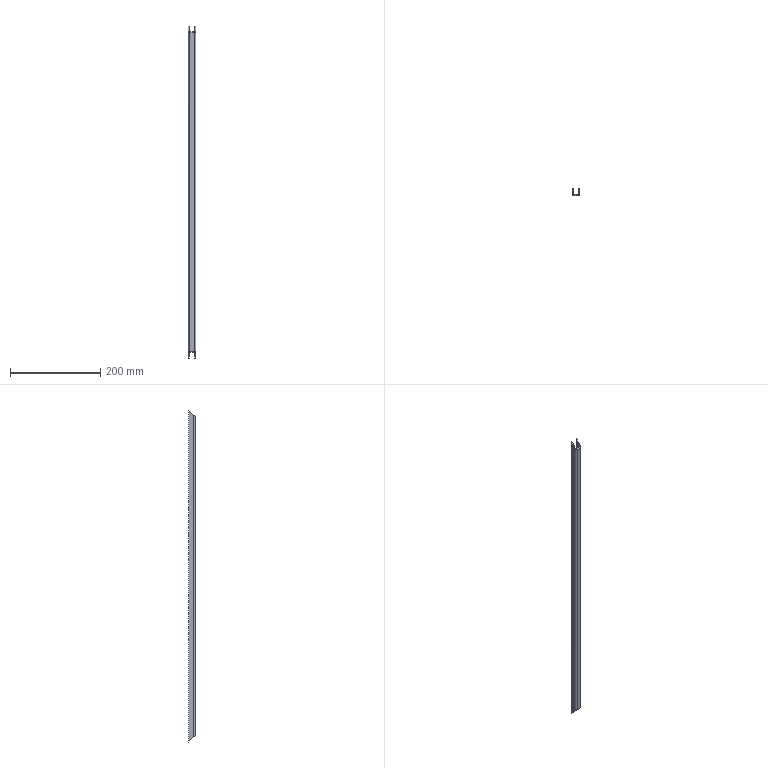Part | STEP file | 1 solid | 14 faces | box 17 x 15 x 736 mm | volume 58634 mm3 | plane 10 | cylinder 4 | commonest cylinder face diameters 3 x2 7 x2
STEP:
#1=CARTESIAN_POINT('',(0.,0.,0.));
#2=DIRECTION('',(0.,0.,1.));
#3=DIRECTION('',(1.,0.,0.));
#4=AXIS2_PLACEMENT_3D('',#1,#2,#3);
#5=CARTESIAN_POINT('',(-6.5,10.,736.));
#6=VERTEX_POINT('',#5);
#7=CARTESIAN_POINT('',(-6.5,10.,0.));
#8=VERTEX_POINT('',#7);
#9=CARTESIAN_POINT('',(-6.5,10.,736.));
#10=DIRECTION('',(0.,0.,-1.));
#11=VECTOR('',#10,1.);
#12=LINE('',#9,#11);
#13=CARTESIAN_POINT('',(-6.5,-5.,736.));
#14=DIRECTION('',(-1.,0.,0.));
#15=DIRECTION('',(0.,0.,1.));
#16=AXIS2_PLACEMENT_3D('',#13,#14,#15);
#17=PLANE('',#16);
#18=CARTESIAN_POINT('',(0.,15.));
#19=DIRECTION('',(-1.,0.));
#20=VECTOR('',#19,1.);
#21=LINE('',#18,#20);
#22=(GEOMETRIC_REPRESENTATION_CONTEXT(2)PARAMETRIC_REPRESENTATION_CONTEXT()REPRESENTATION_CONTEXT('',''));
#23=DEFINITIONAL_REPRESENTATION('',(#21),#22);
#24=PCURVE('',#17,#23);
#25=CARTESIAN_POINT('',(-8.5,10.,736.));
#26=DIRECTION('',(0.,1.,0.));
#27=DIRECTION('',(0.,0.,1.));
#28=AXIS2_PLACEMENT_3D('',#25,#26,#27);
#29=PLANE('',#28);
#30=CARTESIAN_POINT('',(0.,2.));
#31=DIRECTION('',(-1.,0.));
#32=VECTOR('',#31,1.);
#33=LINE('',#30,#32);
#34=(GEOMETRIC_REPRESENTATION_CONTEXT(2)PARAMETRIC_REPRESENTATION_CONTEXT()REPRESENTATION_CONTEXT('',''));
#35=DEFINITIONAL_REPRESENTATION('',(#33),#34);
#36=PCURVE('',#29,#35);
#37=SURFACE_CURVE('',#12,(#24,#36),.PCURVE_S1.);
#38=EDGE_CURVE('',#6,#8,#37,.T.);
#39=ORIENTED_EDGE('',*,*,#38,.F.);
#40=CARTESIAN_POINT('',(-6.5,-1.5,724.5));
#41=VERTEX_POINT('',#40);
#42=CARTESIAN_POINT('',(-6.5,2.5,728.5));
#43=DIRECTION('',(0.,-0.7071,-0.7071));
#44=VECTOR('',#43,1.);
#45=LINE('',#42,#44);
#46=CARTESIAN_POINT('',(-7.5,7.5));
#47=DIRECTION('',(-0.7071,-0.7071));
#48=VECTOR('',#47,1.);
#49=LINE('',#46,#48);
#50=(GEOMETRIC_REPRESENTATION_CONTEXT(2)PARAMETRIC_REPRESENTATION_CONTEXT()REPRESENTATION_CONTEXT('',''));
#51=DEFINITIONAL_REPRESENTATION('',(#49),#50);
#52=PCURVE('',#17,#51);
#53=CARTESIAN_POINT('',(-61.5,10.,736.));
#54=DIRECTION('',(0.,0.7071,-0.7071));
#55=DIRECTION('',(0.,0.7071,0.7071));
#56=AXIS2_PLACEMENT_3D('',#53,#54,#55);
#57=PLANE('',#56);
#58=CARTESIAN_POINT('',(-10.607,55.));
#59=DIRECTION('',(-1.,0.));
#60=VECTOR('',#59,1.);
#61=LINE('',#58,#60);
#62=(GEOMETRIC_REPRESENTATION_CONTEXT(2)PARAMETRIC_REPRESENTATION_CONTEXT()REPRESENTATION_CONTEXT('',''));
#63=DEFINITIONAL_REPRESENTATION('',(#61),#62);
#64=PCURVE('',#57,#63);
#65=SURFACE_CURVE('',#45,(#52,#64),.PCURVE_S1.);
#66=EDGE_CURVE('',#6,#41,#65,.T.);
#67=ORIENTED_EDGE('',*,*,#66,.T.);
#68=CARTESIAN_POINT('',(-6.5,-1.5,11.5));
#69=VERTEX_POINT('',#68);
#70=CARTESIAN_POINT('',(-6.5,-1.5,736.));
#71=DIRECTION('',(0.,0.,-1.));
#72=VECTOR('',#71,1.);
#73=LINE('',#70,#72);
#74=CARTESIAN_POINT('',(0.,3.5));
#75=DIRECTION('',(-1.,0.));
#76=VECTOR('',#75,1.);
#77=LINE('',#74,#76);
#78=(GEOMETRIC_REPRESENTATION_CONTEXT(2)PARAMETRIC_REPRESENTATION_CONTEXT()REPRESENTATION_CONTEXT('',''));
#79=DEFINITIONAL_REPRESENTATION('',(#77),#78);
#80=PCURVE('',#17,#79);
#81=CARTESIAN_POINT('',(-5.,-1.5,736.));
#82=DIRECTION('',(0.,0.,-1.));
#83=DIRECTION('',(-1.,0.,0.));
#84=AXIS2_PLACEMENT_3D('',#81,#82,#83);
#85=CYLINDRICAL_SURFACE('',#84,1.5);
#86=CARTESIAN_POINT('',(6.283,0.));
#87=DIRECTION('',(0.,1.));
#88=VECTOR('',#87,1.);
#89=LINE('',#86,#88);
#90=(GEOMETRIC_REPRESENTATION_CONTEXT(2)PARAMETRIC_REPRESENTATION_CONTEXT()REPRESENTATION_CONTEXT('',''));
#91=DEFINITIONAL_REPRESENTATION('',(#89),#90);
#92=PCURVE('',#85,#91);
#93=SURFACE_CURVE('',#73,(#80,#92),.PCURVE_S1.);
#94=EDGE_CURVE('',#41,#69,#93,.T.);
#95=ORIENTED_EDGE('',*,*,#94,.T.);
#96=CARTESIAN_POINT('',(-6.5,-365.5,375.5));
#97=DIRECTION('',(0.,0.7071,-0.7071));
#98=VECTOR('',#97,1.);
#99=LINE('',#96,#98);
#100=CARTESIAN_POINT('',(-360.5,-360.5));
#101=DIRECTION('',(-0.7071,0.7071));
#102=VECTOR('',#101,1.);
#103=LINE('',#100,#102);
#104=(GEOMETRIC_REPRESENTATION_CONTEXT(2)PARAMETRIC_REPRESENTATION_CONTEXT()REPRESENTATION_CONTEXT('',''));
#105=DEFINITIONAL_REPRESENTATION('',(#103),#104);
#106=PCURVE('',#17,#105);
#107=CARTESIAN_POINT('',(-61.5,10.,0.));
#108=DIRECTION('',(0.,0.7071,0.7071));
#109=DIRECTION('',(0.,-0.7071,0.7071));
#110=AXIS2_PLACEMENT_3D('',#107,#108,#109);
#111=PLANE('',#110);
#112=CARTESIAN_POINT('',(531.037,55.));
#113=DIRECTION('',(-1.,0.));
#114=VECTOR('',#113,1.);
#115=LINE('',#112,#114);
#116=(GEOMETRIC_REPRESENTATION_CONTEXT(2)PARAMETRIC_REPRESENTATION_CONTEXT()REPRESENTATION_CONTEXT('',''));
#117=DEFINITIONAL_REPRESENTATION('',(#115),#116);
#118=PCURVE('',#111,#117);
#119=SURFACE_CURVE('',#99,(#106,#118),.PCURVE_S1.);
#120=EDGE_CURVE('',#69,#8,#119,.T.);
#121=ORIENTED_EDGE('',*,*,#120,.T.);
#122=EDGE_LOOP('',(#39,#67,#95,#121));
#123=FACE_BOUND('',#122,.T.);
#124=ADVANCED_FACE('',(#123),#17,.F.);
#125=CARTESIAN_POINT('',(-8.5,10.,0.));
#126=VERTEX_POINT('',#125);
#127=CARTESIAN_POINT('',(-8.5,10.,0.));
#128=DIRECTION('',(1.,0.,0.));
#129=VECTOR('',#128,1.);
#130=LINE('',#127,#129);
#131=CARTESIAN_POINT('',(-736.,0.));
#132=DIRECTION('',(0.,1.));
#133=VECTOR('',#132,1.);
#134=LINE('',#131,#133);
#135=(GEOMETRIC_REPRESENTATION_CONTEXT(2)PARAMETRIC_REPRESENTATION_CONTEXT()REPRESENTATION_CONTEXT('',''));
#136=DEFINITIONAL_REPRESENTATION('',(#134),#135);
#137=PCURVE('',#29,#136);
#138=CARTESIAN_POINT('',(0.,53.));
#139=DIRECTION('',(0.,1.));
#140=VECTOR('',#139,1.);
#141=LINE('',#138,#140);
#142=(GEOMETRIC_REPRESENTATION_CONTEXT(2)PARAMETRIC_REPRESENTATION_CONTEXT()REPRESENTATION_CONTEXT('',''));
#143=DEFINITIONAL_REPRESENTATION('',(#141),#142);
#144=PCURVE('',#111,#143);
#145=SURFACE_CURVE('',#130,(#137,#144),.PCURVE_S1.);
#146=EDGE_CURVE('',#126,#8,#145,.T.);
#147=ORIENTED_EDGE('',*,*,#146,.F.);
#148=CARTESIAN_POINT('',(-8.5,10.,736.));
#149=VERTEX_POINT('',#148);
#150=CARTESIAN_POINT('',(-8.5,10.,736.));
#151=DIRECTION('',(0.,0.,-1.));
#152=VECTOR('',#151,1.);
#153=LINE('',#150,#152);
#154=CARTESIAN_POINT('',(0.,0.));
#155=DIRECTION('',(-1.,0.));
#156=VECTOR('',#155,1.);
#157=LINE('',#154,#156);
#158=(GEOMETRIC_REPRESENTATION_CONTEXT(2)PARAMETRIC_REPRESENTATION_CONTEXT()REPRESENTATION_CONTEXT('',''));
#159=DEFINITIONAL_REPRESENTATION('',(#157),#158);
#160=PCURVE('',#29,#159);
#161=CARTESIAN_POINT('',(-8.5,-5.,736.));
#162=DIRECTION('',(-1.,0.,0.));
#163=DIRECTION('',(0.,0.,1.));
#164=AXIS2_PLACEMENT_3D('',#161,#162,#163);
#165=PLANE('',#164);
#166=CARTESIAN_POINT('',(0.,15.));
#167=DIRECTION('',(-1.,0.));
#168=VECTOR('',#167,1.);
#169=LINE('',#166,#168);
#170=(GEOMETRIC_REPRESENTATION_CONTEXT(2)PARAMETRIC_REPRESENTATION_CONTEXT()REPRESENTATION_CONTEXT('',''));
#171=DEFINITIONAL_REPRESENTATION('',(#169),#170);
#172=PCURVE('',#165,#171);
#173=SURFACE_CURVE('',#153,(#160,#172),.PCURVE_S1.);
#174=EDGE_CURVE('',#149,#126,#173,.T.);
#175=ORIENTED_EDGE('',*,*,#174,.F.);
#176=CARTESIAN_POINT('',(-8.5,10.,736.));
#177=DIRECTION('',(1.,0.,0.));
#178=VECTOR('',#177,1.);
#179=LINE('',#176,#178);
#180=CARTESIAN_POINT('',(0.,0.));
#181=DIRECTION('',(0.,1.));
#182=VECTOR('',#181,1.);
#183=LINE('',#180,#182);
#184=(GEOMETRIC_REPRESENTATION_CONTEXT(2)PARAMETRIC_REPRESENTATION_CONTEXT()REPRESENTATION_CONTEXT('',''));
#185=DEFINITIONAL_REPRESENTATION('',(#183),#184);
#186=PCURVE('',#29,#185);
#187=CARTESIAN_POINT('',(0.,53.));
#188=DIRECTION('',(0.,1.));
#189=VECTOR('',#188,1.);
#190=LINE('',#187,#189);
#191=(GEOMETRIC_REPRESENTATION_CONTEXT(2)PARAMETRIC_REPRESENTATION_CONTEXT()REPRESENTATION_CONTEXT('',''));
#192=DEFINITIONAL_REPRESENTATION('',(#190),#191);
#193=PCURVE('',#57,#192);
#194=SURFACE_CURVE('',#179,(#186,#193),.PCURVE_S1.);
#195=EDGE_CURVE('',#149,#6,#194,.T.);
#196=ORIENTED_EDGE('',*,*,#195,.T.);
#197=ORIENTED_EDGE('',*,*,#38,.T.);
#198=EDGE_LOOP('',(#147,#175,#196,#197));
#199=FACE_BOUND('',#198,.T.);
#200=ADVANCED_FACE('',(#199),#29,.T.);
#201=CARTESIAN_POINT('',(-8.5,-1.5,724.5));
#202=VERTEX_POINT('',#201);
#203=CARTESIAN_POINT('',(-8.5,2.5,728.5));
#204=DIRECTION('',(0.,-0.7071,-0.7071));
#205=VECTOR('',#204,1.);
#206=LINE('',#203,#205);
#207=CARTESIAN_POINT('',(-7.5,7.5));
#208=DIRECTION('',(-0.7071,-0.7071));
#209=VECTOR('',#208,1.);
#210=LINE('',#207,#209);
#211=(GEOMETRIC_REPRESENTATION_CONTEXT(2)PARAMETRIC_REPRESENTATION_CONTEXT()REPRESENTATION_CONTEXT('',''));
#212=DEFINITIONAL_REPRESENTATION('',(#210),#211);
#213=PCURVE('',#165,#212);
#214=CARTESIAN_POINT('',(-10.607,53.));
#215=DIRECTION('',(-1.,0.));
#216=VECTOR('',#215,1.);
#217=LINE('',#214,#216);
#218=(GEOMETRIC_REPRESENTATION_CONTEXT(2)PARAMETRIC_REPRESENTATION_CONTEXT()REPRESENTATION_CONTEXT('',''));
#219=DEFINITIONAL_REPRESENTATION('',(#217),#218);
#220=PCURVE('',#57,#219);
#221=SURFACE_CURVE('',#206,(#213,#220),.PCURVE_S1.);
#222=EDGE_CURVE('',#149,#202,#221,.T.);
#223=ORIENTED_EDGE('',*,*,#222,.F.);
#224=ORIENTED_EDGE('',*,*,#174,.T.);
#225=CARTESIAN_POINT('',(-8.5,-1.5,11.5));
#226=VERTEX_POINT('',#225);
#227=CARTESIAN_POINT('',(-8.5,-365.5,375.5));
#228=DIRECTION('',(0.,0.7071,-0.7071));
#229=VECTOR('',#228,1.);
#230=LINE('',#227,#229);
#231=CARTESIAN_POINT('',(-360.5,-360.5));
#232=DIRECTION('',(-0.7071,0.7071));
#233=VECTOR('',#232,1.);
#234=LINE('',#231,#233);
#235=(GEOMETRIC_REPRESENTATION_CONTEXT(2)PARAMETRIC_REPRESENTATION_CONTEXT()REPRESENTATION_CONTEXT('',''));
#236=DEFINITIONAL_REPRESENTATION('',(#234),#235);
#237=PCURVE('',#165,#236);
#238=CARTESIAN_POINT('',(531.037,53.));
#239=DIRECTION('',(-1.,0.));
#240=VECTOR('',#239,1.);
#241=LINE('',#238,#240);
#242=(GEOMETRIC_REPRESENTATION_CONTEXT(2)PARAMETRIC_REPRESENTATION_CONTEXT()REPRESENTATION_CONTEXT('',''));
#243=DEFINITIONAL_REPRESENTATION('',(#241),#242);
#244=PCURVE('',#111,#243);
#245=SURFACE_CURVE('',#230,(#237,#244),.PCURVE_S1.);
#246=EDGE_CURVE('',#226,#126,#245,.T.);
#247=ORIENTED_EDGE('',*,*,#246,.F.);
#248=CARTESIAN_POINT('',(-8.5,-1.5,736.));
#249=DIRECTION('',(0.,0.,-1.));
#250=VECTOR('',#249,1.);
#251=LINE('',#248,#250);
#252=CARTESIAN_POINT('',(0.,3.5));
#253=DIRECTION('',(-1.,0.));
#254=VECTOR('',#253,1.);
#255=LINE('',#252,#254);
#256=(GEOMETRIC_REPRESENTATION_CONTEXT(2)PARAMETRIC_REPRESENTATION_CONTEXT()REPRESENTATION_CONTEXT('',''));
#257=DEFINITIONAL_REPRESENTATION('',(#255),#256);
#258=PCURVE('',#165,#257);
#259=CARTESIAN_POINT('',(-5.,-1.5,736.));
#260=DIRECTION('',(0.,0.,-1.));
#261=DIRECTION('',(-1.,0.,0.));
#262=AXIS2_PLACEMENT_3D('',#259,#260,#261);
#263=CYLINDRICAL_SURFACE('',#262,3.5);
#264=CARTESIAN_POINT('',(6.283,0.));
#265=DIRECTION('',(0.,1.));
#266=VECTOR('',#265,1.);
#267=LINE('',#264,#266);
#268=(GEOMETRIC_REPRESENTATION_CONTEXT(2)PARAMETRIC_REPRESENTATION_CONTEXT()REPRESENTATION_CONTEXT('',''));
#269=DEFINITIONAL_REPRESENTATION('',(#267),#268);
#270=PCURVE('',#263,#269);
#271=SURFACE_CURVE('',#251,(#258,#270),.PCURVE_S1.);
#272=EDGE_CURVE('',#202,#226,#271,.T.);
#273=ORIENTED_EDGE('',*,*,#272,.F.);
#274=EDGE_LOOP('',(#223,#224,#247,#273));
#275=FACE_BOUND('',#274,.T.);
#276=ADVANCED_FACE('',(#275),#165,.T.);
#277=CARTESIAN_POINT('',(-5.,-5.,721.));
#278=VERTEX_POINT('',#277);
#279=CARTESIAN_POINT('',(-8.5,-1.5,724.5));
#280=CARTESIAN_POINT('',(-8.5,-3.55,722.45));
#281=CARTESIAN_POINT('',(-7.05,-5.,721.));
#282=CARTESIAN_POINT('',(-5.,-5.,721.));
#283=(BOUNDED_CURVE()B_SPLINE_CURVE(3,(#279,#280,#281,#282),.UNSPECIFIED.,.F.,.F.)B_SPLINE_CURVE_WITH_KNOTS((4,4),(4.712,6.283),.PIECEWISE_BEZIER_KNOTS.)CURVE()GEOMETRIC_REPRESENTATION_ITEM()RATIONAL_B_SPLINE_CURVE((1.,0.8047,0.8047,1.))REPRESENTATION_ITEM(''));
#284=CARTESIAN_POINT('',(6.283,11.5));
#285=CARTESIAN_POINT('',(6.262,11.575));
#286=CARTESIAN_POINT('',(6.218,11.727));
#287=CARTESIAN_POINT('',(6.152,11.96));
#288=CARTESIAN_POINT('',(6.083,12.196));
#289=CARTESIAN_POINT('',(6.013,12.433));
#290=CARTESIAN_POINT('',(5.942,12.671));
#291=CARTESIAN_POINT('',(5.87,12.906));
#292=CARTESIAN_POINT('',(5.797,13.137));
#293=CARTESIAN_POINT('',(5.723,13.362));
#294=CARTESIAN_POINT('',(5.648,13.578));
#295=CARTESIAN_POINT('',(5.573,13.784));
#296=CARTESIAN_POINT('',(5.498,13.977));
#297=CARTESIAN_POINT('',(5.422,14.157));
#298=CARTESIAN_POINT('',(5.347,14.32));
#299=CARTESIAN_POINT('',(5.273,14.468));
#300=CARTESIAN_POINT('',(5.199,14.597));
#301=CARTESIAN_POINT('',(5.125,14.709));
#302=CARTESIAN_POINT('',(5.053,14.802));
#303=CARTESIAN_POINT('',(4.982,14.876));
#304=CARTESIAN_POINT('',(4.912,14.933));
#305=CARTESIAN_POINT('',(4.844,14.972));
#306=CARTESIAN_POINT('',(4.777,14.995));
#307=CARTESIAN_POINT('',(4.734,15.));
#308=CARTESIAN_POINT('',(4.712,15.));
#309=B_SPLINE_CURVE_WITH_KNOTS('',3,(#284,#285,#286,#287,#288,#289,#290,#291,#292,#293,#294,#295,#296,#297,#298,#299,#300,#301,#302,#303,#304,#305,#306,#307,#308),.UNSPECIFIED.,.F.,.F.,(4,1,1,1,1,1,1,1,1,1,1,1,1,1,1,1,1,1,1,1,1,1,4),(4.712,4.784,4.855,4.927,4.998,5.069,5.141,5.212,5.284,5.355,5.426,5.498,5.569,5.641,5.712,5.783,5.855,5.926,5.998,6.069,6.14,6.212,6.283),.QUASI_UNIFORM_KNOTS.);
#310=(GEOMETRIC_REPRESENTATION_CONTEXT(2)PARAMETRIC_REPRESENTATION_CONTEXT()REPRESENTATION_CONTEXT('',''));
#311=DEFINITIONAL_REPRESENTATION('',(#309),#310);
#312=PCURVE('',#263,#311);
#313=CARTESIAN_POINT('',(-16.263,53.));
#314=CARTESIAN_POINT('',(-19.163,53.));
#315=CARTESIAN_POINT('',(-21.213,54.45));
#316=CARTESIAN_POINT('',(-21.213,56.5));
#317=(BOUNDED_CURVE()B_SPLINE_CURVE(3,(#313,#314,#315,#316),.UNSPECIFIED.,.F.,.F.)B_SPLINE_CURVE_WITH_KNOTS((4,4),(4.712,6.283),.PIECEWISE_BEZIER_KNOTS.)CURVE()GEOMETRIC_REPRESENTATION_ITEM()RATIONAL_B_SPLINE_CURVE((1.,0.8047,0.8047,1.))REPRESENTATION_ITEM(''));
#318=(GEOMETRIC_REPRESENTATION_CONTEXT(2)PARAMETRIC_REPRESENTATION_CONTEXT()REPRESENTATION_CONTEXT('',''));
#319=DEFINITIONAL_REPRESENTATION('',(#317),#318);
#320=PCURVE('',#57,#319);
#321=SURFACE_CURVE('',#283,(#312,#320),.PCURVE_S1.);
#322=EDGE_CURVE('',#202,#278,#321,.T.);
#323=ORIENTED_EDGE('',*,*,#322,.F.);
#324=ORIENTED_EDGE('',*,*,#272,.T.);
#325=CARTESIAN_POINT('',(-5.,-5.,15.));
#326=VERTEX_POINT('',#325);
#327=CARTESIAN_POINT('',(-5.,-5.,15.));
#328=CARTESIAN_POINT('',(-7.05,-5.,15.));
#329=CARTESIAN_POINT('',(-8.5,-3.55,13.55));
#330=CARTESIAN_POINT('',(-8.5,-1.5,11.5));
#331=(BOUNDED_CURVE()B_SPLINE_CURVE(3,(#327,#328,#329,#330),.UNSPECIFIED.,.F.,.F.)B_SPLINE_CURVE_WITH_KNOTS((4,4),(3.142,4.712),.PIECEWISE_BEZIER_KNOTS.)CURVE()GEOMETRIC_REPRESENTATION_ITEM()RATIONAL_B_SPLINE_CURVE((1.,0.8047,0.8047,1.))REPRESENTATION_ITEM(''));
#332=CARTESIAN_POINT('',(4.712,721.));
#333=CARTESIAN_POINT('',(4.734,721.));
#334=CARTESIAN_POINT('',(4.777,721.005));
#335=CARTESIAN_POINT('',(4.844,721.028));
#336=CARTESIAN_POINT('',(4.912,721.067));
#337=CARTESIAN_POINT('',(4.982,721.124));
#338=CARTESIAN_POINT('',(5.053,721.198));
#339=CARTESIAN_POINT('',(5.125,721.291));
#340=CARTESIAN_POINT('',(5.199,721.403));
#341=CARTESIAN_POINT('',(5.273,721.532));
#342=CARTESIAN_POINT('',(5.347,721.68));
#343=CARTESIAN_POINT('',(5.422,721.843));
#344=CARTESIAN_POINT('',(5.498,722.023));
#345=CARTESIAN_POINT('',(5.573,722.216));
#346=CARTESIAN_POINT('',(5.648,722.422));
#347=CARTESIAN_POINT('',(5.723,722.638));
#348=CARTESIAN_POINT('',(5.797,722.863));
#349=CARTESIAN_POINT('',(5.87,723.094));
#350=CARTESIAN_POINT('',(5.942,723.329));
#351=CARTESIAN_POINT('',(6.013,723.567));
#352=CARTESIAN_POINT('',(6.083,723.804));
#353=CARTESIAN_POINT('',(6.152,724.04));
#354=CARTESIAN_POINT('',(6.218,724.273));
#355=CARTESIAN_POINT('',(6.262,724.425));
#356=CARTESIAN_POINT('',(6.283,724.5));
#357=B_SPLINE_CURVE_WITH_KNOTS('',3,(#332,#333,#334,#335,#336,#337,#338,#339,#340,#341,#342,#343,#344,#345,#346,#347,#348,#349,#350,#351,#352,#353,#354,#355,#356),.UNSPECIFIED.,.F.,.F.,(4,1,1,1,1,1,1,1,1,1,1,1,1,1,1,1,1,1,1,1,1,1,4),(3.142,3.213,3.284,3.356,3.427,3.499,3.57,3.641,3.713,3.784,3.856,3.927,3.998,4.07,4.141,4.213,4.284,4.355,4.427,4.498,4.57,4.641,4.712),.QUASI_UNIFORM_KNOTS.);
#358=(GEOMETRIC_REPRESENTATION_CONTEXT(2)PARAMETRIC_REPRESENTATION_CONTEXT()REPRESENTATION_CONTEXT('',''));
#359=DEFINITIONAL_REPRESENTATION('',(#357),#358);
#360=PCURVE('',#263,#359);
#361=CARTESIAN_POINT('',(21.213,56.5));
#362=CARTESIAN_POINT('',(21.213,54.45));
#363=CARTESIAN_POINT('',(19.163,53.));
#364=CARTESIAN_POINT('',(16.263,53.));
#365=(BOUNDED_CURVE()B_SPLINE_CURVE(3,(#361,#362,#363,#364),.UNSPECIFIED.,.F.,.F.)B_SPLINE_CURVE_WITH_KNOTS((4,4),(3.142,4.712),.PIECEWISE_BEZIER_KNOTS.)CURVE()GEOMETRIC_REPRESENTATION_ITEM()RATIONAL_B_SPLINE_CURVE((1.,0.8047,0.8047,1.))REPRESENTATION_ITEM(''));
#366=(GEOMETRIC_REPRESENTATION_CONTEXT(2)PARAMETRIC_REPRESENTATION_CONTEXT()REPRESENTATION_CONTEXT('',''));
#367=DEFINITIONAL_REPRESENTATION('',(#365),#366);
#368=PCURVE('',#111,#367);
#369=SURFACE_CURVE('',#331,(#360,#368),.PCURVE_S1.);
#370=EDGE_CURVE('',#326,#226,#369,.T.);
#371=ORIENTED_EDGE('',*,*,#370,.F.);
#372=CARTESIAN_POINT('',(-5.,-5.,736.));
#373=DIRECTION('',(0.,0.,-1.));
#374=VECTOR('',#373,1.);
#375=LINE('',#372,#374);
#376=CARTESIAN_POINT('',(4.712,0.));
#377=DIRECTION('',(0.,1.));
#378=VECTOR('',#377,1.);
#379=LINE('',#376,#378);
#380=(GEOMETRIC_REPRESENTATION_CONTEXT(2)PARAMETRIC_REPRESENTATION_CONTEXT()REPRESENTATION_CONTEXT('',''));
#381=DEFINITIONAL_REPRESENTATION('',(#379),#380);
#382=PCURVE('',#263,#381);
#383=CARTESIAN_POINT('',(-8.5,-5.,736.));
#384=DIRECTION('',(0.,-1.,0.));
#385=DIRECTION('',(0.,0.,-1.));
#386=AXIS2_PLACEMENT_3D('',#383,#384,#385);
#387=PLANE('',#386);
#388=CARTESIAN_POINT('',(0.,3.5));
#389=DIRECTION('',(1.,0.));
#390=VECTOR('',#389,1.);
#391=LINE('',#388,#390);
#392=(GEOMETRIC_REPRESENTATION_CONTEXT(2)PARAMETRIC_REPRESENTATION_CONTEXT()REPRESENTATION_CONTEXT('',''));
#393=DEFINITIONAL_REPRESENTATION('',(#391),#392);
#394=PCURVE('',#387,#393);
#395=SURFACE_CURVE('',#375,(#382,#394),.PCURVE_S1.);
#396=EDGE_CURVE('',#278,#326,#395,.T.);
#397=ORIENTED_EDGE('',*,*,#396,.F.);
#398=EDGE_LOOP('',(#323,#324,#371,#397));
#399=FACE_BOUND('',#398,.T.);
#400=ADVANCED_FACE('',(#399),#263,.T.);
#401=CARTESIAN_POINT('',(5.,-5.,721.));
#402=VERTEX_POINT('',#401);
#403=CARTESIAN_POINT('',(-61.5,-5.,721.));
#404=DIRECTION('',(1.,0.,0.));
#405=VECTOR('',#404,1.);
#406=LINE('',#403,#405);
#407=CARTESIAN_POINT('',(15.,-53.));
#408=DIRECTION('',(0.,1.));
#409=VECTOR('',#408,1.);
#410=LINE('',#407,#409);
#411=(GEOMETRIC_REPRESENTATION_CONTEXT(2)PARAMETRIC_REPRESENTATION_CONTEXT()REPRESENTATION_CONTEXT('',''));
#412=DEFINITIONAL_REPRESENTATION('',(#410),#411);
#413=PCURVE('',#387,#412);
#414=CARTESIAN_POINT('',(-21.213,0.));
#415=DIRECTION('',(0.,1.));
#416=VECTOR('',#415,1.);
#417=LINE('',#414,#416);
#418=(GEOMETRIC_REPRESENTATION_CONTEXT(2)PARAMETRIC_REPRESENTATION_CONTEXT()REPRESENTATION_CONTEXT('',''));
#419=DEFINITIONAL_REPRESENTATION('',(#417),#418);
#420=PCURVE('',#57,#419);
#421=SURFACE_CURVE('',#406,(#413,#420),.PCURVE_S1.);
#422=EDGE_CURVE('',#278,#402,#421,.T.);
#423=ORIENTED_EDGE('',*,*,#422,.F.);
#424=ORIENTED_EDGE('',*,*,#396,.T.);
#425=CARTESIAN_POINT('',(5.,-5.,15.));
#426=VERTEX_POINT('',#425);
#427=CARTESIAN_POINT('',(-61.5,-5.,15.));
#428=DIRECTION('',(1.,0.,0.));
#429=VECTOR('',#428,1.);
#430=LINE('',#427,#429);
#431=CARTESIAN_POINT('',(721.,-53.));
#432=DIRECTION('',(0.,1.));
#433=VECTOR('',#432,1.);
#434=LINE('',#431,#433);
#435=(GEOMETRIC_REPRESENTATION_CONTEXT(2)PARAMETRIC_REPRESENTATION_CONTEXT()REPRESENTATION_CONTEXT('',''));
#436=DEFINITIONAL_REPRESENTATION('',(#434),#435);
#437=PCURVE('',#387,#436);
#438=CARTESIAN_POINT('',(21.213,0.));
#439=DIRECTION('',(0.,1.));
#440=VECTOR('',#439,1.);
#441=LINE('',#438,#440);
#442=(GEOMETRIC_REPRESENTATION_CONTEXT(2)PARAMETRIC_REPRESENTATION_CONTEXT()REPRESENTATION_CONTEXT('',''));
#443=DEFINITIONAL_REPRESENTATION('',(#441),#442);
#444=PCURVE('',#111,#443);
#445=SURFACE_CURVE('',#430,(#437,#444),.PCURVE_S1.);
#446=EDGE_CURVE('',#326,#426,#445,.T.);
#447=ORIENTED_EDGE('',*,*,#446,.T.);
#448=CARTESIAN_POINT('',(5.,-5.,736.));
#449=DIRECTION('',(0.,0.,-1.));
#450=VECTOR('',#449,1.);
#451=LINE('',#448,#450);
#452=CARTESIAN_POINT('',(0.,13.5));
#453=DIRECTION('',(1.,0.));
#454=VECTOR('',#453,1.);
#455=LINE('',#452,#454);
#456=(GEOMETRIC_REPRESENTATION_CONTEXT(2)PARAMETRIC_REPRESENTATION_CONTEXT()REPRESENTATION_CONTEXT('',''));
#457=DEFINITIONAL_REPRESENTATION('',(#455),#456);
#458=PCURVE('',#387,#457);
#459=CARTESIAN_POINT('',(5.,-1.5,736.));
#460=DIRECTION('',(0.,0.,-1.));
#461=DIRECTION('',(-1.,0.,0.));
#462=AXIS2_PLACEMENT_3D('',#459,#460,#461);
#463=CYLINDRICAL_SURFACE('',#462,3.5);
#464=CARTESIAN_POINT('',(4.712,0.));
#465=DIRECTION('',(0.,1.));
#466=VECTOR('',#465,1.);
#467=LINE('',#464,#466);
#468=(GEOMETRIC_REPRESENTATION_CONTEXT(2)PARAMETRIC_REPRESENTATION_CONTEXT()REPRESENTATION_CONTEXT('',''));
#469=DEFINITIONAL_REPRESENTATION('',(#467),#468);
#470=PCURVE('',#463,#469);
#471=SURFACE_CURVE('',#451,(#458,#470),.PCURVE_S1.);
#472=EDGE_CURVE('',#402,#426,#471,.T.);
#473=ORIENTED_EDGE('',*,*,#472,.F.);
#474=EDGE_LOOP('',(#423,#424,#447,#473));
#475=FACE_BOUND('',#474,.T.);
#476=ADVANCED_FACE('',(#475),#387,.T.);
#477=CARTESIAN_POINT('',(8.5,-1.5,724.5));
#478=VERTEX_POINT('',#477);
#479=CARTESIAN_POINT('',(5.,-5.,721.));
#480=CARTESIAN_POINT('',(7.05,-5.,721.));
#481=CARTESIAN_POINT('',(8.5,-3.55,722.45));
#482=CARTESIAN_POINT('',(8.5,-1.5,724.5));
#483=(BOUNDED_CURVE()B_SPLINE_CURVE(3,(#479,#480,#481,#482),.UNSPECIFIED.,.F.,.F.)B_SPLINE_CURVE_WITH_KNOTS((4,4),(0.,1.571),.PIECEWISE_BEZIER_KNOTS.)CURVE()GEOMETRIC_REPRESENTATION_ITEM()RATIONAL_B_SPLINE_CURVE((1.,0.8047,0.8047,1.))REPRESENTATION_ITEM(''));
#484=CARTESIAN_POINT('',(4.712,15.));
#485=CARTESIAN_POINT('',(4.691,15.));
#486=CARTESIAN_POINT('',(4.648,14.995));
#487=CARTESIAN_POINT('',(4.581,14.972));
#488=CARTESIAN_POINT('',(4.512,14.933));
#489=CARTESIAN_POINT('',(4.443,14.876));
#490=CARTESIAN_POINT('',(4.372,14.802));
#491=CARTESIAN_POINT('',(4.299,14.709));
#492=CARTESIAN_POINT('',(4.226,14.597));
#493=CARTESIAN_POINT('',(4.152,14.468));
#494=CARTESIAN_POINT('',(4.077,14.32));
#495=CARTESIAN_POINT('',(4.002,14.157));
#496=CARTESIAN_POINT('',(3.927,13.977));
#497=CARTESIAN_POINT('',(3.852,13.784));
#498=CARTESIAN_POINT('',(3.777,13.578));
#499=CARTESIAN_POINT('',(3.702,13.362));
#500=CARTESIAN_POINT('',(3.628,13.137));
#501=CARTESIAN_POINT('',(3.555,12.906));
#502=CARTESIAN_POINT('',(3.482,12.671));
#503=CARTESIAN_POINT('',(3.411,12.433));
#504=CARTESIAN_POINT('',(3.342,12.196));
#505=CARTESIAN_POINT('',(3.273,11.96));
#506=CARTESIAN_POINT('',(3.206,11.727));
#507=CARTESIAN_POINT('',(3.163,11.575));
#508=CARTESIAN_POINT('',(3.142,11.5));
#509=B_SPLINE_CURVE_WITH_KNOTS('',3,(#484,#485,#486,#487,#488,#489,#490,#491,#492,#493,#494,#495,#496,#497,#498,#499,#500,#501,#502,#503,#504,#505,#506,#507,#508),.UNSPECIFIED.,.F.,.F.,(4,1,1,1,1,1,1,1,1,1,1,1,1,1,1,1,1,1,1,1,1,1,4),(0.,0.0714,0.1428,0.2142,0.2856,0.357,0.4284,0.4998,0.5712,0.6426,0.714,0.7854,0.8568,0.9282,0.9996,1.071,1.142,1.214,1.285,1.357,1.428,1.499,1.571),.QUASI_UNIFORM_KNOTS.);
#510=(GEOMETRIC_REPRESENTATION_CONTEXT(2)PARAMETRIC_REPRESENTATION_CONTEXT()REPRESENTATION_CONTEXT('',''));
#511=DEFINITIONAL_REPRESENTATION('',(#509),#510);
#512=PCURVE('',#463,#511);
#513=CARTESIAN_POINT('',(-21.213,66.5));
#514=CARTESIAN_POINT('',(-21.213,68.55));
#515=CARTESIAN_POINT('',(-19.163,70.));
#516=CARTESIAN_POINT('',(-16.263,70.));
#517=(BOUNDED_CURVE()B_SPLINE_CURVE(3,(#513,#514,#515,#516),.UNSPECIFIED.,.F.,.F.)B_SPLINE_CURVE_WITH_KNOTS((4,4),(0.,1.571),.PIECEWISE_BEZIER_KNOTS.)CURVE()GEOMETRIC_REPRESENTATION_ITEM()RATIONAL_B_SPLINE_CURVE((1.,0.8047,0.8047,1.))REPRESENTATION_ITEM(''));
#518=(GEOMETRIC_REPRESENTATION_CONTEXT(2)PARAMETRIC_REPRESENTATION_CONTEXT()REPRESENTATION_CONTEXT('',''));
#519=DEFINITIONAL_REPRESENTATION('',(#517),#518);
#520=PCURVE('',#57,#519);
#521=SURFACE_CURVE('',#483,(#512,#520),.PCURVE_S1.);
#522=EDGE_CURVE('',#402,#478,#521,.T.);
#523=ORIENTED_EDGE('',*,*,#522,.F.);
#524=ORIENTED_EDGE('',*,*,#472,.T.);
#525=CARTESIAN_POINT('',(8.5,-1.5,11.5));
#526=VERTEX_POINT('',#525);
#527=CARTESIAN_POINT('',(8.5,-1.5,11.5));
#528=CARTESIAN_POINT('',(8.5,-3.55,13.55));
#529=CARTESIAN_POINT('',(7.05,-5.,15.));
#530=CARTESIAN_POINT('',(5.,-5.,15.));
#531=(BOUNDED_CURVE()B_SPLINE_CURVE(3,(#527,#528,#529,#530),.UNSPECIFIED.,.F.,.F.)B_SPLINE_CURVE_WITH_KNOTS((4,4),(1.571,3.142),.PIECEWISE_BEZIER_KNOTS.)CURVE()GEOMETRIC_REPRESENTATION_ITEM()RATIONAL_B_SPLINE_CURVE((1.,0.8047,0.8047,1.))REPRESENTATION_ITEM(''));
#532=CARTESIAN_POINT('',(3.142,724.5));
#533=CARTESIAN_POINT('',(3.163,724.425));
#534=CARTESIAN_POINT('',(3.206,724.273));
#535=CARTESIAN_POINT('',(3.273,724.04));
#536=CARTESIAN_POINT('',(3.342,723.804));
#537=CARTESIAN_POINT('',(3.411,723.567));
#538=CARTESIAN_POINT('',(3.482,723.329));
#539=CARTESIAN_POINT('',(3.555,723.094));
#540=CARTESIAN_POINT('',(3.628,722.863));
#541=CARTESIAN_POINT('',(3.702,722.638));
#542=CARTESIAN_POINT('',(3.777,722.422));
#543=CARTESIAN_POINT('',(3.852,722.216));
#544=CARTESIAN_POINT('',(3.927,722.023));
#545=CARTESIAN_POINT('',(4.002,721.843));
#546=CARTESIAN_POINT('',(4.077,721.68));
#547=CARTESIAN_POINT('',(4.152,721.532));
#548=CARTESIAN_POINT('',(4.226,721.403));
#549=CARTESIAN_POINT('',(4.299,721.291));
#550=CARTESIAN_POINT('',(4.372,721.198));
#551=CARTESIAN_POINT('',(4.443,721.124));
#552=CARTESIAN_POINT('',(4.512,721.067));
#553=CARTESIAN_POINT('',(4.581,721.028));
#554=CARTESIAN_POINT('',(4.648,721.005));
#555=CARTESIAN_POINT('',(4.691,721.));
#556=CARTESIAN_POINT('',(4.712,721.));
#557=B_SPLINE_CURVE_WITH_KNOTS('',3,(#532,#533,#534,#535,#536,#537,#538,#539,#540,#541,#542,#543,#544,#545,#546,#547,#548,#549,#550,#551,#552,#553,#554,#555,#556),.UNSPECIFIED.,.F.,.F.,(4,1,1,1,1,1,1,1,1,1,1,1,1,1,1,1,1,1,1,1,1,1,4),(1.571,1.642,1.714,1.785,1.856,1.928,1.999,2.071,2.142,2.213,2.285,2.356,2.428,2.499,2.57,2.642,2.713,2.785,2.856,2.927,2.999,3.07,3.142),.QUASI_UNIFORM_KNOTS.);
#558=(GEOMETRIC_REPRESENTATION_CONTEXT(2)PARAMETRIC_REPRESENTATION_CONTEXT()REPRESENTATION_CONTEXT('',''));
#559=DEFINITIONAL_REPRESENTATION('',(#557),#558);
#560=PCURVE('',#463,#559);
#561=CARTESIAN_POINT('',(16.263,70.));
#562=CARTESIAN_POINT('',(19.163,70.));
#563=CARTESIAN_POINT('',(21.213,68.55));
#564=CARTESIAN_POINT('',(21.213,66.5));
#565=(BOUNDED_CURVE()B_SPLINE_CURVE(3,(#561,#562,#563,#564),.UNSPECIFIED.,.F.,.F.)B_SPLINE_CURVE_WITH_KNOTS((4,4),(1.571,3.142),.PIECEWISE_BEZIER_KNOTS.)CURVE()GEOMETRIC_REPRESENTATION_ITEM()RATIONAL_B_SPLINE_CURVE((1.,0.8047,0.8047,1.))REPRESENTATION_ITEM(''));
#566=(GEOMETRIC_REPRESENTATION_CONTEXT(2)PARAMETRIC_REPRESENTATION_CONTEXT()REPRESENTATION_CONTEXT('',''));
#567=DEFINITIONAL_REPRESENTATION('',(#565),#566);
#568=PCURVE('',#111,#567);
#569=SURFACE_CURVE('',#531,(#560,#568),.PCURVE_S1.);
#570=EDGE_CURVE('',#526,#426,#569,.T.);
#571=ORIENTED_EDGE('',*,*,#570,.F.);
#572=CARTESIAN_POINT('',(8.5,-1.5,736.));
#573=DIRECTION('',(0.,0.,-1.));
#574=VECTOR('',#573,1.);
#575=LINE('',#572,#574);
#576=CARTESIAN_POINT('',(3.142,0.));
#577=DIRECTION('',(0.,1.));
#578=VECTOR('',#577,1.);
#579=LINE('',#576,#578);
#580=(GEOMETRIC_REPRESENTATION_CONTEXT(2)PARAMETRIC_REPRESENTATION_CONTEXT()REPRESENTATION_CONTEXT('',''));
#581=DEFINITIONAL_REPRESENTATION('',(#579),#580);
#582=PCURVE('',#463,#581);
#583=CARTESIAN_POINT('',(8.5,-5.,736.));
#584=DIRECTION('',(1.,0.,0.));
#585=DIRECTION('',(0.,0.,-1.));
#586=AXIS2_PLACEMENT_3D('',#583,#584,#585);
#587=PLANE('',#586);
#588=CARTESIAN_POINT('',(0.,3.5));
#589=DIRECTION('',(1.,0.));
#590=VECTOR('',#589,1.);
#591=LINE('',#588,#590);
#592=(GEOMETRIC_REPRESENTATION_CONTEXT(2)PARAMETRIC_REPRESENTATION_CONTEXT()REPRESENTATION_CONTEXT('',''));
#593=DEFINITIONAL_REPRESENTATION('',(#591),#592);
#594=PCURVE('',#587,#593);
#595=SURFACE_CURVE('',#575,(#582,#594),.PCURVE_S1.);
#596=EDGE_CURVE('',#478,#526,#595,.T.);
#597=ORIENTED_EDGE('',*,*,#596,.F.);
#598=EDGE_LOOP('',(#523,#524,#571,#597));
#599=FACE_BOUND('',#598,.T.);
#600=ADVANCED_FACE('',(#599),#463,.T.);
#601=CARTESIAN_POINT('',(8.5,10.,736.));
#602=VERTEX_POINT('',#601);
#603=CARTESIAN_POINT('',(8.5,10.,736.));
#604=DIRECTION('',(0.,0.7071,0.7071));
#605=VECTOR('',#604,1.);
#606=LINE('',#603,#605);
#607=CARTESIAN_POINT('',(0.,15.));
#608=DIRECTION('',(-0.7071,0.7071));
#609=VECTOR('',#608,1.);
#610=LINE('',#607,#609);
#611=(GEOMETRIC_REPRESENTATION_CONTEXT(2)PARAMETRIC_REPRESENTATION_CONTEXT()REPRESENTATION_CONTEXT('',''));
#612=DEFINITIONAL_REPRESENTATION('',(#610),#611);
#613=PCURVE('',#587,#612);
#614=CARTESIAN_POINT('',(0.,70.));
#615=DIRECTION('',(1.,0.));
#616=VECTOR('',#615,1.);
#617=LINE('',#614,#616);
#618=(GEOMETRIC_REPRESENTATION_CONTEXT(2)PARAMETRIC_REPRESENTATION_CONTEXT()REPRESENTATION_CONTEXT('',''));
#619=DEFINITIONAL_REPRESENTATION('',(#617),#618);
#620=PCURVE('',#57,#619);
#621=SURFACE_CURVE('',#606,(#613,#620),.PCURVE_S1.);
#622=EDGE_CURVE('',#478,#602,#621,.T.);
#623=ORIENTED_EDGE('',*,*,#622,.F.);
#624=ORIENTED_EDGE('',*,*,#596,.T.);
#625=CARTESIAN_POINT('',(8.5,10.,0.));
#626=VERTEX_POINT('',#625);
#627=CARTESIAN_POINT('',(8.5,10.,0.));
#628=DIRECTION('',(0.,-0.7071,0.7071));
#629=VECTOR('',#628,1.);
#630=LINE('',#627,#629);
#631=CARTESIAN_POINT('',(736.,15.));
#632=DIRECTION('',(-0.7071,-0.7071));
#633=VECTOR('',#632,1.);
#634=LINE('',#631,#633);
#635=(GEOMETRIC_REPRESENTATION_CONTEXT(2)PARAMETRIC_REPRESENTATION_CONTEXT()REPRESENTATION_CONTEXT('',''));
#636=DEFINITIONAL_REPRESENTATION('',(#634),#635);
#637=PCURVE('',#587,#636);
#638=CARTESIAN_POINT('',(0.,70.));
#639=DIRECTION('',(1.,0.));
#640=VECTOR('',#639,1.);
#641=LINE('',#638,#640);
#642=(GEOMETRIC_REPRESENTATION_CONTEXT(2)PARAMETRIC_REPRESENTATION_CONTEXT()REPRESENTATION_CONTEXT('',''));
#643=DEFINITIONAL_REPRESENTATION('',(#641),#642);
#644=PCURVE('',#111,#643);
#645=SURFACE_CURVE('',#630,(#637,#644),.PCURVE_S1.);
#646=EDGE_CURVE('',#626,#526,#645,.T.);
#647=ORIENTED_EDGE('',*,*,#646,.F.);
#648=CARTESIAN_POINT('',(8.5,10.,736.));
#649=DIRECTION('',(0.,0.,-1.));
#650=VECTOR('',#649,1.);
#651=LINE('',#648,#650);
#652=CARTESIAN_POINT('',(0.,15.));
#653=DIRECTION('',(1.,0.));
#654=VECTOR('',#653,1.);
#655=LINE('',#652,#654);
#656=(GEOMETRIC_REPRESENTATION_CONTEXT(2)PARAMETRIC_REPRESENTATION_CONTEXT()REPRESENTATION_CONTEXT('',''));
#657=DEFINITIONAL_REPRESENTATION('',(#655),#656);
#658=PCURVE('',#587,#657);
#659=CARTESIAN_POINT('',(6.5,10.,736.));
#660=DIRECTION('',(0.,1.,0.));
#661=DIRECTION('',(0.,0.,1.));
#662=AXIS2_PLACEMENT_3D('',#659,#660,#661);
#663=PLANE('',#662);
#664=CARTESIAN_POINT('',(0.,2.));
#665=DIRECTION('',(-1.,0.));
#666=VECTOR('',#665,1.);
#667=LINE('',#664,#666);
#668=(GEOMETRIC_REPRESENTATION_CONTEXT(2)PARAMETRIC_REPRESENTATION_CONTEXT()REPRESENTATION_CONTEXT('',''));
#669=DEFINITIONAL_REPRESENTATION('',(#667),#668);
#670=PCURVE('',#663,#669);
#671=SURFACE_CURVE('',#651,(#658,#670),.PCURVE_S1.);
#672=EDGE_CURVE('',#602,#626,#671,.T.);
#673=ORIENTED_EDGE('',*,*,#672,.F.);
#674=EDGE_LOOP('',(#623,#624,#647,#673));
#675=FACE_BOUND('',#674,.T.);
#676=ADVANCED_FACE('',(#675),#587,.T.);
#677=CARTESIAN_POINT('',(6.5,10.,0.));
#678=VERTEX_POINT('',#677);
#679=CARTESIAN_POINT('',(6.5,10.,0.));
#680=DIRECTION('',(1.,0.,0.));
#681=VECTOR('',#680,1.);
#682=LINE('',#679,#681);
#683=CARTESIAN_POINT('',(-736.,0.));
#684=DIRECTION('',(0.,1.));
#685=VECTOR('',#684,1.);
#686=LINE('',#683,#685);
#687=(GEOMETRIC_REPRESENTATION_CONTEXT(2)PARAMETRIC_REPRESENTATION_CONTEXT()REPRESENTATION_CONTEXT('',''));
#688=DEFINITIONAL_REPRESENTATION('',(#686),#687);
#689=PCURVE('',#663,#688);
#690=CARTESIAN_POINT('',(0.,68.));
#691=DIRECTION('',(0.,1.));
#692=VECTOR('',#691,1.);
#693=LINE('',#690,#692);
#694=(GEOMETRIC_REPRESENTATION_CONTEXT(2)PARAMETRIC_REPRESENTATION_CONTEXT()REPRESENTATION_CONTEXT('',''));
#695=DEFINITIONAL_REPRESENTATION('',(#693),#694);
#696=PCURVE('',#111,#695);
#697=SURFACE_CURVE('',#682,(#689,#696),.PCURVE_S1.);
#698=EDGE_CURVE('',#678,#626,#697,.T.);
#699=ORIENTED_EDGE('',*,*,#698,.F.);
#700=CARTESIAN_POINT('',(6.5,10.,736.));
#701=VERTEX_POINT('',#700);
#702=CARTESIAN_POINT('',(6.5,10.,736.));
#703=DIRECTION('',(0.,0.,-1.));
#704=VECTOR('',#703,1.);
#705=LINE('',#702,#704);
#706=CARTESIAN_POINT('',(0.,0.));
#707=DIRECTION('',(-1.,0.));
#708=VECTOR('',#707,1.);
#709=LINE('',#706,#708);
#710=(GEOMETRIC_REPRESENTATION_CONTEXT(2)PARAMETRIC_REPRESENTATION_CONTEXT()REPRESENTATION_CONTEXT('',''));
#711=DEFINITIONAL_REPRESENTATION('',(#709),#710);
#712=PCURVE('',#663,#711);
#713=CARTESIAN_POINT('',(6.5,-5.,736.));
#714=DIRECTION('',(1.,0.,0.));
#715=DIRECTION('',(0.,0.,-1.));
#716=AXIS2_PLACEMENT_3D('',#713,#714,#715);
#717=PLANE('',#716);
#718=CARTESIAN_POINT('',(0.,15.));
#719=DIRECTION('',(1.,0.));
#720=VECTOR('',#719,1.);
#721=LINE('',#718,#720);
#722=(GEOMETRIC_REPRESENTATION_CONTEXT(2)PARAMETRIC_REPRESENTATION_CONTEXT()REPRESENTATION_CONTEXT('',''));
#723=DEFINITIONAL_REPRESENTATION('',(#721),#722);
#724=PCURVE('',#717,#723);
#725=SURFACE_CURVE('',#705,(#712,#724),.PCURVE_S1.);
#726=EDGE_CURVE('',#701,#678,#725,.T.);
#727=ORIENTED_EDGE('',*,*,#726,.F.);
#728=CARTESIAN_POINT('',(6.5,10.,736.));
#729=DIRECTION('',(1.,0.,0.));
#730=VECTOR('',#729,1.);
#731=LINE('',#728,#730);
#732=CARTESIAN_POINT('',(0.,0.));
#733=DIRECTION('',(0.,1.));
#734=VECTOR('',#733,1.);
#735=LINE('',#732,#734);
#736=(GEOMETRIC_REPRESENTATION_CONTEXT(2)PARAMETRIC_REPRESENTATION_CONTEXT()REPRESENTATION_CONTEXT('',''));
#737=DEFINITIONAL_REPRESENTATION('',(#735),#736);
#738=PCURVE('',#663,#737);
#739=CARTESIAN_POINT('',(0.,68.));
#740=DIRECTION('',(0.,1.));
#741=VECTOR('',#740,1.);
#742=LINE('',#739,#741);
#743=(GEOMETRIC_REPRESENTATION_CONTEXT(2)PARAMETRIC_REPRESENTATION_CONTEXT()REPRESENTATION_CONTEXT('',''));
#744=DEFINITIONAL_REPRESENTATION('',(#742),#743);
#745=PCURVE('',#57,#744);
#746=SURFACE_CURVE('',#731,(#738,#745),.PCURVE_S1.);
#747=EDGE_CURVE('',#701,#602,#746,.T.);
#748=ORIENTED_EDGE('',*,*,#747,.T.);
#749=ORIENTED_EDGE('',*,*,#672,.T.);
#750=EDGE_LOOP('',(#699,#727,#748,#749));
#751=FACE_BOUND('',#750,.T.);
#752=ADVANCED_FACE('',(#751),#663,.T.);
#753=CARTESIAN_POINT('',(6.5,-1.5,724.5));
#754=VERTEX_POINT('',#753);
#755=CARTESIAN_POINT('',(6.5,-1.5,11.5));
#756=VERTEX_POINT('',#755);
#757=CARTESIAN_POINT('',(6.5,-1.5,736.));
#758=DIRECTION('',(0.,0.,-1.));
#759=VECTOR('',#758,1.);
#760=LINE('',#757,#759);
#761=CARTESIAN_POINT('',(0.,3.5));
#762=DIRECTION('',(1.,0.));
#763=VECTOR('',#762,1.);
#764=LINE('',#761,#763);
#765=(GEOMETRIC_REPRESENTATION_CONTEXT(2)PARAMETRIC_REPRESENTATION_CONTEXT()REPRESENTATION_CONTEXT('',''));
#766=DEFINITIONAL_REPRESENTATION('',(#764),#765);
#767=PCURVE('',#717,#766);
#768=CARTESIAN_POINT('',(5.,-1.5,736.));
#769=DIRECTION('',(0.,0.,-1.));
#770=DIRECTION('',(-1.,0.,0.));
#771=AXIS2_PLACEMENT_3D('',#768,#769,#770);
#772=CYLINDRICAL_SURFACE('',#771,1.5);
#773=CARTESIAN_POINT('',(3.142,0.));
#774=DIRECTION('',(0.,1.));
#775=VECTOR('',#774,1.);
#776=LINE('',#773,#775);
#777=(GEOMETRIC_REPRESENTATION_CONTEXT(2)PARAMETRIC_REPRESENTATION_CONTEXT()REPRESENTATION_CONTEXT('',''));
#778=DEFINITIONAL_REPRESENTATION('',(#776),#777);
#779=PCURVE('',#772,#778);
#780=SURFACE_CURVE('',#760,(#767,#779),.PCURVE_S1.);
#781=EDGE_CURVE('',#754,#756,#780,.T.);
#782=ORIENTED_EDGE('',*,*,#781,.F.);
#783=CARTESIAN_POINT('',(6.5,2.5,728.5));
#784=DIRECTION('',(0.,0.7071,0.7071));
#785=VECTOR('',#784,1.);
#786=LINE('',#783,#785);
#787=CARTESIAN_POINT('',(7.5,7.5));
#788=DIRECTION('',(-0.7071,0.7071));
#789=VECTOR('',#788,1.);
#790=LINE('',#787,#789);
#791=(GEOMETRIC_REPRESENTATION_CONTEXT(2)PARAMETRIC_REPRESENTATION_CONTEXT()REPRESENTATION_CONTEXT('',''));
#792=DEFINITIONAL_REPRESENTATION('',(#790),#791);
#793=PCURVE('',#717,#792);
#794=CARTESIAN_POINT('',(-10.607,68.));
#795=DIRECTION('',(1.,0.));
#796=VECTOR('',#795,1.);
#797=LINE('',#794,#796);
#798=(GEOMETRIC_REPRESENTATION_CONTEXT(2)PARAMETRIC_REPRESENTATION_CONTEXT()REPRESENTATION_CONTEXT('',''));
#799=DEFINITIONAL_REPRESENTATION('',(#797),#798);
#800=PCURVE('',#57,#799);
#801=SURFACE_CURVE('',#786,(#793,#800),.PCURVE_S1.);
#802=EDGE_CURVE('',#754,#701,#801,.T.);
#803=ORIENTED_EDGE('',*,*,#802,.T.);
#804=ORIENTED_EDGE('',*,*,#726,.T.);
#805=CARTESIAN_POINT('',(6.5,-365.5,375.5));
#806=DIRECTION('',(0.,-0.7071,0.7071));
#807=VECTOR('',#806,1.);
#808=LINE('',#805,#807);
#809=CARTESIAN_POINT('',(360.5,-360.5));
#810=DIRECTION('',(-0.7071,-0.7071));
#811=VECTOR('',#810,1.);
#812=LINE('',#809,#811);
#813=(GEOMETRIC_REPRESENTATION_CONTEXT(2)PARAMETRIC_REPRESENTATION_CONTEXT()REPRESENTATION_CONTEXT('',''));
#814=DEFINITIONAL_REPRESENTATION('',(#812),#813);
#815=PCURVE('',#717,#814);
#816=CARTESIAN_POINT('',(531.037,68.));
#817=DIRECTION('',(1.,0.));
#818=VECTOR('',#817,1.);
#819=LINE('',#816,#818);
#820=(GEOMETRIC_REPRESENTATION_CONTEXT(2)PARAMETRIC_REPRESENTATION_CONTEXT()REPRESENTATION_CONTEXT('',''));
#821=DEFINITIONAL_REPRESENTATION('',(#819),#820);
#822=PCURVE('',#111,#821);
#823=SURFACE_CURVE('',#808,(#815,#822),.PCURVE_S1.);
#824=EDGE_CURVE('',#678,#756,#823,.T.);
#825=ORIENTED_EDGE('',*,*,#824,.T.);
#826=EDGE_LOOP('',(#782,#803,#804,#825));
#827=FACE_BOUND('',#826,.T.);
#828=ADVANCED_FACE('',(#827),#717,.F.);
#829=CARTESIAN_POINT('',(5.,-3.,13.));
#830=VERTEX_POINT('',#829);
#831=CARTESIAN_POINT('',(6.5,-1.5,11.5));
#832=CARTESIAN_POINT('',(6.5,-2.379,12.379));
#833=CARTESIAN_POINT('',(5.879,-3.,13.));
#834=CARTESIAN_POINT('',(5.,-3.,13.));
#835=(BOUNDED_CURVE()B_SPLINE_CURVE(3,(#831,#832,#833,#834),.UNSPECIFIED.,.F.,.F.)B_SPLINE_CURVE_WITH_KNOTS((4,4),(1.571,3.142),.PIECEWISE_BEZIER_KNOTS.)CURVE()GEOMETRIC_REPRESENTATION_ITEM()RATIONAL_B_SPLINE_CURVE((1.,0.8047,0.8047,1.))REPRESENTATION_ITEM(''));
#836=CARTESIAN_POINT('',(3.142,724.5));
#837=CARTESIAN_POINT('',(3.163,724.468));
#838=CARTESIAN_POINT('',(3.206,724.403));
#839=CARTESIAN_POINT('',(3.273,724.303));
#840=CARTESIAN_POINT('',(3.342,724.202));
#841=CARTESIAN_POINT('',(3.411,724.1));
#842=CARTESIAN_POINT('',(3.482,723.998));
#843=CARTESIAN_POINT('',(3.555,723.897));
#844=CARTESIAN_POINT('',(3.628,723.798));
#845=CARTESIAN_POINT('',(3.702,723.702));
#846=CARTESIAN_POINT('',(3.777,723.609));
#847=CARTESIAN_POINT('',(3.852,723.521));
#848=CARTESIAN_POINT('',(3.927,723.438));
#849=CARTESIAN_POINT('',(4.002,723.361));
#850=CARTESIAN_POINT('',(4.077,723.291));
#851=CARTESIAN_POINT('',(4.152,723.228));
#852=CARTESIAN_POINT('',(4.226,723.173));
#853=CARTESIAN_POINT('',(4.299,723.125));
#854=CARTESIAN_POINT('',(4.372,723.085));
#855=CARTESIAN_POINT('',(4.443,723.053));
#856=CARTESIAN_POINT('',(4.512,723.029));
#857=CARTESIAN_POINT('',(4.581,723.012));
#858=CARTESIAN_POINT('',(4.648,723.002));
#859=CARTESIAN_POINT('',(4.691,723.));
#860=CARTESIAN_POINT('',(4.712,723.));
#861=B_SPLINE_CURVE_WITH_KNOTS('',3,(#836,#837,#838,#839,#840,#841,#842,#843,#844,#845,#846,#847,#848,#849,#850,#851,#852,#853,#854,#855,#856,#857,#858,#859,#860),.UNSPECIFIED.,.F.,.F.,(4,1,1,1,1,1,1,1,1,1,1,1,1,1,1,1,1,1,1,1,1,1,4),(1.571,1.642,1.714,1.785,1.856,1.928,1.999,2.071,2.142,2.213,2.285,2.356,2.428,2.499,2.57,2.642,2.713,2.785,2.856,2.927,2.999,3.07,3.142),.QUASI_UNIFORM_KNOTS.);
#862=(GEOMETRIC_REPRESENTATION_CONTEXT(2)PARAMETRIC_REPRESENTATION_CONTEXT()REPRESENTATION_CONTEXT('',''));
#863=DEFINITIONAL_REPRESENTATION('',(#861),#862);
#864=PCURVE('',#772,#863);
#865=CARTESIAN_POINT('',(16.263,68.));
#866=CARTESIAN_POINT('',(17.506,68.));
#867=CARTESIAN_POINT('',(18.385,67.379));
#868=CARTESIAN_POINT('',(18.385,66.5));
#869=(BOUNDED_CURVE()B_SPLINE_CURVE(3,(#865,#866,#867,#868),.UNSPECIFIED.,.F.,.F.)B_SPLINE_CURVE_WITH_KNOTS((4,4),(1.571,3.142),.PIECEWISE_BEZIER_KNOTS.)CURVE()GEOMETRIC_REPRESENTATION_ITEM()RATIONAL_B_SPLINE_CURVE((1.,0.8047,0.8047,1.))REPRESENTATION_ITEM(''));
#870=(GEOMETRIC_REPRESENTATION_CONTEXT(2)PARAMETRIC_REPRESENTATION_CONTEXT()REPRESENTATION_CONTEXT('',''));
#871=DEFINITIONAL_REPRESENTATION('',(#869),#870);
#872=PCURVE('',#111,#871);
#873=SURFACE_CURVE('',#835,(#864,#872),.PCURVE_S1.);
#874=EDGE_CURVE('',#756,#830,#873,.T.);
#875=ORIENTED_EDGE('',*,*,#874,.F.);
#876=ORIENTED_EDGE('',*,*,#781,.F.);
#877=CARTESIAN_POINT('',(5.,-3.,723.));
#878=VERTEX_POINT('',#877);
#879=CARTESIAN_POINT('',(5.,-3.,723.));
#880=CARTESIAN_POINT('',(5.879,-3.,723.));
#881=CARTESIAN_POINT('',(6.5,-2.379,723.621));
#882=CARTESIAN_POINT('',(6.5,-1.5,724.5));
#883=(BOUNDED_CURVE()B_SPLINE_CURVE(3,(#879,#880,#881,#882),.UNSPECIFIED.,.F.,.F.)B_SPLINE_CURVE_WITH_KNOTS((4,4),(0.,1.571),.PIECEWISE_BEZIER_KNOTS.)CURVE()GEOMETRIC_REPRESENTATION_ITEM()RATIONAL_B_SPLINE_CURVE((1.,0.8047,0.8047,1.))REPRESENTATION_ITEM(''));
#884=CARTESIAN_POINT('',(4.712,13.));
#885=CARTESIAN_POINT('',(4.691,13.));
#886=CARTESIAN_POINT('',(4.648,12.998));
#887=CARTESIAN_POINT('',(4.581,12.988));
#888=CARTESIAN_POINT('',(4.512,12.971));
#889=CARTESIAN_POINT('',(4.443,12.947));
#890=CARTESIAN_POINT('',(4.372,12.915));
#891=CARTESIAN_POINT('',(4.299,12.875));
#892=CARTESIAN_POINT('',(4.226,12.827));
#893=CARTESIAN_POINT('',(4.152,12.772));
#894=CARTESIAN_POINT('',(4.077,12.709));
#895=CARTESIAN_POINT('',(4.002,12.639));
#896=CARTESIAN_POINT('',(3.927,12.562));
#897=CARTESIAN_POINT('',(3.852,12.479));
#898=CARTESIAN_POINT('',(3.777,12.391));
#899=CARTESIAN_POINT('',(3.702,12.298));
#900=CARTESIAN_POINT('',(3.628,12.202));
#901=CARTESIAN_POINT('',(3.555,12.103));
#902=CARTESIAN_POINT('',(3.482,12.002));
#903=CARTESIAN_POINT('',(3.411,11.9));
#904=CARTESIAN_POINT('',(3.342,11.798));
#905=CARTESIAN_POINT('',(3.273,11.697));
#906=CARTESIAN_POINT('',(3.206,11.597));
#907=CARTESIAN_POINT('',(3.163,11.532));
#908=CARTESIAN_POINT('',(3.142,11.5));
#909=B_SPLINE_CURVE_WITH_KNOTS('',3,(#884,#885,#886,#887,#888,#889,#890,#891,#892,#893,#894,#895,#896,#897,#898,#899,#900,#901,#902,#903,#904,#905,#906,#907,#908),.UNSPECIFIED.,.F.,.F.,(4,1,1,1,1,1,1,1,1,1,1,1,1,1,1,1,1,1,1,1,1,1,4),(0.,0.0714,0.1428,0.2142,0.2856,0.357,0.4284,0.4998,0.5712,0.6426,0.714,0.7854,0.8568,0.9282,0.9996,1.071,1.142,1.214,1.285,1.357,1.428,1.499,1.571),.QUASI_UNIFORM_KNOTS.);
#910=(GEOMETRIC_REPRESENTATION_CONTEXT(2)PARAMETRIC_REPRESENTATION_CONTEXT()REPRESENTATION_CONTEXT('',''));
#911=DEFINITIONAL_REPRESENTATION('',(#909),#910);
#912=PCURVE('',#772,#911);
#913=CARTESIAN_POINT('',(-18.385,66.5));
#914=CARTESIAN_POINT('',(-18.385,67.379));
#915=CARTESIAN_POINT('',(-17.506,68.));
#916=CARTESIAN_POINT('',(-16.263,68.));
#917=(BOUNDED_CURVE()B_SPLINE_CURVE(3,(#913,#914,#915,#916),.UNSPECIFIED.,.F.,.F.)B_SPLINE_CURVE_WITH_KNOTS((4,4),(0.,1.571),.PIECEWISE_BEZIER_KNOTS.)CURVE()GEOMETRIC_REPRESENTATION_ITEM()RATIONAL_B_SPLINE_CURVE((1.,0.8047,0.8047,1.))REPRESENTATION_ITEM(''));
#918=(GEOMETRIC_REPRESENTATION_CONTEXT(2)PARAMETRIC_REPRESENTATION_CONTEXT()REPRESENTATION_CONTEXT('',''));
#919=DEFINITIONAL_REPRESENTATION('',(#917),#918);
#920=PCURVE('',#57,#919);
#921=SURFACE_CURVE('',#883,(#912,#920),.PCURVE_S1.);
#922=EDGE_CURVE('',#878,#754,#921,.T.);
#923=ORIENTED_EDGE('',*,*,#922,.F.);
#924=CARTESIAN_POINT('',(5.,-3.,736.));
#925=DIRECTION('',(0.,0.,-1.));
#926=VECTOR('',#925,1.);
#927=LINE('',#924,#926);
#928=CARTESIAN_POINT('',(4.712,0.));
#929=DIRECTION('',(0.,1.));
#930=VECTOR('',#929,1.);
#931=LINE('',#928,#930);
#932=(GEOMETRIC_REPRESENTATION_CONTEXT(2)PARAMETRIC_REPRESENTATION_CONTEXT()REPRESENTATION_CONTEXT('',''));
#933=DEFINITIONAL_REPRESENTATION('',(#931),#932);
#934=PCURVE('',#772,#933);
#935=CARTESIAN_POINT('',(-8.5,-3.,736.));
#936=DIRECTION('',(0.,-1.,0.));
#937=DIRECTION('',(0.,0.,-1.));
#938=AXIS2_PLACEMENT_3D('',#935,#936,#937);
#939=PLANE('',#938);
#940=CARTESIAN_POINT('',(0.,13.5));
#941=DIRECTION('',(1.,0.));
#942=VECTOR('',#941,1.);
#943=LINE('',#940,#942);
#944=(GEOMETRIC_REPRESENTATION_CONTEXT(2)PARAMETRIC_REPRESENTATION_CONTEXT()REPRESENTATION_CONTEXT('',''));
#945=DEFINITIONAL_REPRESENTATION('',(#943),#944);
#946=PCURVE('',#939,#945);
#947=SURFACE_CURVE('',#927,(#934,#946),.PCURVE_S1.);
#948=EDGE_CURVE('',#878,#830,#947,.T.);
#949=ORIENTED_EDGE('',*,*,#948,.T.);
#950=EDGE_LOOP('',(#875,#876,#923,#949));
#951=FACE_BOUND('',#950,.F.);
#952=ADVANCED_FACE('',(#951),#772,.F.);
#953=CARTESIAN_POINT('',(-5.,-3.,723.));
#954=VERTEX_POINT('',#953);
#955=CARTESIAN_POINT('',(-5.,-3.,13.));
#956=VERTEX_POINT('',#955);
#957=CARTESIAN_POINT('',(-5.,-3.,736.));
#958=DIRECTION('',(0.,0.,-1.));
#959=VECTOR('',#958,1.);
#960=LINE('',#957,#959);
#961=CARTESIAN_POINT('',(0.,3.5));
#962=DIRECTION('',(1.,0.));
#963=VECTOR('',#962,1.);
#964=LINE('',#961,#963);
#965=(GEOMETRIC_REPRESENTATION_CONTEXT(2)PARAMETRIC_REPRESENTATION_CONTEXT()REPRESENTATION_CONTEXT('',''));
#966=DEFINITIONAL_REPRESENTATION('',(#964),#965);
#967=PCURVE('',#939,#966);
#968=CARTESIAN_POINT('',(4.712,0.));
#969=DIRECTION('',(0.,1.));
#970=VECTOR('',#969,1.);
#971=LINE('',#968,#970);
#972=(GEOMETRIC_REPRESENTATION_CONTEXT(2)PARAMETRIC_REPRESENTATION_CONTEXT()REPRESENTATION_CONTEXT('',''));
#973=DEFINITIONAL_REPRESENTATION('',(#971),#972);
#974=PCURVE('',#85,#973);
#975=SURFACE_CURVE('',#960,(#967,#974),.PCURVE_S1.);
#976=EDGE_CURVE('',#954,#956,#975,.T.);
#977=ORIENTED_EDGE('',*,*,#976,.F.);
#978=CARTESIAN_POINT('',(-8.5,-3.,723.));
#979=DIRECTION('',(1.,0.,0.));
#980=VECTOR('',#979,1.);
#981=LINE('',#978,#980);
#982=CARTESIAN_POINT('',(13.,0.));
#983=DIRECTION('',(0.,1.));
#984=VECTOR('',#983,1.);
#985=LINE('',#982,#984);
#986=(GEOMETRIC_REPRESENTATION_CONTEXT(2)PARAMETRIC_REPRESENTATION_CONTEXT()REPRESENTATION_CONTEXT('',''));
#987=DEFINITIONAL_REPRESENTATION('',(#985),#986);
#988=PCURVE('',#939,#987);
#989=CARTESIAN_POINT('',(-18.385,53.));
#990=DIRECTION('',(0.,1.));
#991=VECTOR('',#990,1.);
#992=LINE('',#989,#991);
#993=(GEOMETRIC_REPRESENTATION_CONTEXT(2)PARAMETRIC_REPRESENTATION_CONTEXT()REPRESENTATION_CONTEXT('',''));
#994=DEFINITIONAL_REPRESENTATION('',(#992),#993);
#995=PCURVE('',#57,#994);
#996=SURFACE_CURVE('',#981,(#988,#995),.PCURVE_S1.);
#997=EDGE_CURVE('',#954,#878,#996,.T.);
#998=ORIENTED_EDGE('',*,*,#997,.T.);
#999=ORIENTED_EDGE('',*,*,#948,.T.);
#1000=CARTESIAN_POINT('',(-8.5,-3.,13.));
#1001=DIRECTION('',(-1.,0.,0.));
#1002=VECTOR('',#1001,1.);
#1003=LINE('',#1000,#1002);
#1004=CARTESIAN_POINT('',(723.,0.));
#1005=DIRECTION('',(0.,-1.));
#1006=VECTOR('',#1005,1.);
#1007=LINE('',#1004,#1006);
#1008=(GEOMETRIC_REPRESENTATION_CONTEXT(2)PARAMETRIC_REPRESENTATION_CONTEXT()REPRESENTATION_CONTEXT('',''));
#1009=DEFINITIONAL_REPRESENTATION('',(#1007),#1008);
#1010=PCURVE('',#939,#1009);
#1011=CARTESIAN_POINT('',(18.385,53.));
#1012=DIRECTION('',(0.,-1.));
#1013=VECTOR('',#1012,1.);
#1014=LINE('',#1011,#1013);
#1015=(GEOMETRIC_REPRESENTATION_CONTEXT(2)PARAMETRIC_REPRESENTATION_CONTEXT()REPRESENTATION_CONTEXT('',''));
#1016=DEFINITIONAL_REPRESENTATION('',(#1014),#1015);
#1017=PCURVE('',#111,#1016);
#1018=SURFACE_CURVE('',#1003,(#1010,#1017),.PCURVE_S1.);
#1019=EDGE_CURVE('',#830,#956,#1018,.T.);
#1020=ORIENTED_EDGE('',*,*,#1019,.T.);
#1021=EDGE_LOOP('',(#977,#998,#999,#1020));
#1022=FACE_BOUND('',#1021,.T.);
#1023=ADVANCED_FACE('',(#1022),#939,.F.);
#1024=CARTESIAN_POINT('',(-5.,-3.,13.));
#1025=CARTESIAN_POINT('',(-5.879,-3.,13.));
#1026=CARTESIAN_POINT('',(-6.5,-2.379,12.379));
#1027=CARTESIAN_POINT('',(-6.5,-1.5,11.5));
#1028=(BOUNDED_CURVE()B_SPLINE_CURVE(3,(#1024,#1025,#1026,#1027),.UNSPECIFIED.,.F.,.F.)B_SPLINE_CURVE_WITH_KNOTS((4,4),(3.142,4.712),.PIECEWISE_BEZIER_KNOTS.)CURVE()GEOMETRIC_REPRESENTATION_ITEM()RATIONAL_B_SPLINE_CURVE((1.,0.8047,0.8047,1.))REPRESENTATION_ITEM(''));
#1029=CARTESIAN_POINT('',(4.712,723.));
#1030=CARTESIAN_POINT('',(4.734,723.));
#1031=CARTESIAN_POINT('',(4.777,723.002));
#1032=CARTESIAN_POINT('',(4.844,723.012));
#1033=CARTESIAN_POINT('',(4.912,723.029));
#1034=CARTESIAN_POINT('',(4.982,723.053));
#1035=CARTESIAN_POINT('',(5.053,723.085));
#1036=CARTESIAN_POINT('',(5.125,723.125));
#1037=CARTESIAN_POINT('',(5.199,723.173));
#1038=CARTESIAN_POINT('',(5.273,723.228));
#1039=CARTESIAN_POINT('',(5.347,723.291));
#1040=CARTESIAN_POINT('',(5.422,723.361));
#1041=CARTESIAN_POINT('',(5.498,723.438));
#1042=CARTESIAN_POINT('',(5.573,723.521));
#1043=CARTESIAN_POINT('',(5.648,723.609));
#1044=CARTESIAN_POINT('',(5.723,723.702));
#1045=CARTESIAN_POINT('',(5.797,723.798));
#1046=CARTESIAN_POINT('',(5.87,723.897));
#1047=CARTESIAN_POINT('',(5.942,723.998));
#1048=CARTESIAN_POINT('',(6.013,724.1));
#1049=CARTESIAN_POINT('',(6.083,724.202));
#1050=CARTESIAN_POINT('',(6.152,724.303));
#1051=CARTESIAN_POINT('',(6.218,724.403));
#1052=CARTESIAN_POINT('',(6.262,724.468));
#1053=CARTESIAN_POINT('',(6.283,724.5));
#1054=B_SPLINE_CURVE_WITH_KNOTS('',3,(#1029,#1030,#1031,#1032,#1033,#1034,#1035,#1036,#1037,#1038,#1039,#1040,#1041,#1042,#1043,#1044,#1045,#1046,#1047,#1048,#1049,#1050,#1051,#1052,#1053),.UNSPECIFIED.,.F.,.F.,(4,1,1,1,1,1,1,1,1,1,1,1,1,1,1,1,1,1,1,1,1,1,4),(3.142,3.213,3.284,3.356,3.427,3.499,3.57,3.641,3.713,3.784,3.856,3.927,3.998,4.07,4.141,4.213,4.284,4.355,4.427,4.498,4.57,4.641,4.712),.QUASI_UNIFORM_KNOTS.);
#1055=(GEOMETRIC_REPRESENTATION_CONTEXT(2)PARAMETRIC_REPRESENTATION_CONTEXT()REPRESENTATION_CONTEXT('',''));
#1056=DEFINITIONAL_REPRESENTATION('',(#1054),#1055);
#1057=PCURVE('',#85,#1056);
#1058=CARTESIAN_POINT('',(18.385,56.5));
#1059=CARTESIAN_POINT('',(18.385,55.621));
#1060=CARTESIAN_POINT('',(17.506,55.));
#1061=CARTESIAN_POINT('',(16.263,55.));
#1062=(BOUNDED_CURVE()B_SPLINE_CURVE(3,(#1058,#1059,#1060,#1061),.UNSPECIFIED.,.F.,.F.)B_SPLINE_CURVE_WITH_KNOTS((4,4),(3.142,4.712),.PIECEWISE_BEZIER_KNOTS.)CURVE()GEOMETRIC_REPRESENTATION_ITEM()RATIONAL_B_SPLINE_CURVE((1.,0.8047,0.8047,1.))REPRESENTATION_ITEM(''));
#1063=(GEOMETRIC_REPRESENTATION_CONTEXT(2)PARAMETRIC_REPRESENTATION_CONTEXT()REPRESENTATION_CONTEXT('',''));
#1064=DEFINITIONAL_REPRESENTATION('',(#1062),#1063);
#1065=PCURVE('',#111,#1064);
#1066=SURFACE_CURVE('',#1028,(#1057,#1065),.PCURVE_S1.);
#1067=EDGE_CURVE('',#956,#69,#1066,.T.);
#1068=ORIENTED_EDGE('',*,*,#1067,.F.);
#1069=ORIENTED_EDGE('',*,*,#976,.F.);
#1070=CARTESIAN_POINT('',(-6.5,-1.5,724.5));
#1071=CARTESIAN_POINT('',(-6.5,-2.379,723.621));
#1072=CARTESIAN_POINT('',(-5.879,-3.,723.));
#1073=CARTESIAN_POINT('',(-5.,-3.,723.));
#1074=(BOUNDED_CURVE()B_SPLINE_CURVE(3,(#1070,#1071,#1072,#1073),.UNSPECIFIED.,.F.,.F.)B_SPLINE_CURVE_WITH_KNOTS((4,4),(4.712,6.283),.PIECEWISE_BEZIER_KNOTS.)CURVE()GEOMETRIC_REPRESENTATION_ITEM()RATIONAL_B_SPLINE_CURVE((1.,0.8047,0.8047,1.))REPRESENTATION_ITEM(''));
#1075=CARTESIAN_POINT('',(6.283,11.5));
#1076=CARTESIAN_POINT('',(6.262,11.532));
#1077=CARTESIAN_POINT('',(6.218,11.597));
#1078=CARTESIAN_POINT('',(6.152,11.697));
#1079=CARTESIAN_POINT('',(6.083,11.798));
#1080=CARTESIAN_POINT('',(6.013,11.9));
#1081=CARTESIAN_POINT('',(5.942,12.002));
#1082=CARTESIAN_POINT('',(5.87,12.103));
#1083=CARTESIAN_POINT('',(5.797,12.202));
#1084=CARTESIAN_POINT('',(5.723,12.298));
#1085=CARTESIAN_POINT('',(5.648,12.391));
#1086=CARTESIAN_POINT('',(5.573,12.479));
#1087=CARTESIAN_POINT('',(5.498,12.562));
#1088=CARTESIAN_POINT('',(5.422,12.639));
#1089=CARTESIAN_POINT('',(5.347,12.709));
#1090=CARTESIAN_POINT('',(5.273,12.772));
#1091=CARTESIAN_POINT('',(5.199,12.827));
#1092=CARTESIAN_POINT('',(5.125,12.875));
#1093=CARTESIAN_POINT('',(5.053,12.915));
#1094=CARTESIAN_POINT('',(4.982,12.947));
#1095=CARTESIAN_POINT('',(4.912,12.971));
#1096=CARTESIAN_POINT('',(4.844,12.988));
#1097=CARTESIAN_POINT('',(4.777,12.998));
#1098=CARTESIAN_POINT('',(4.734,13.));
#1099=CARTESIAN_POINT('',(4.712,13.));
#1100=B_SPLINE_CURVE_WITH_KNOTS('',3,(#1075,#1076,#1077,#1078,#1079,#1080,#1081,#1082,#1083,#1084,#1085,#1086,#1087,#1088,#1089,#1090,#1091,#1092,#1093,#1094,#1095,#1096,#1097,#1098,#1099),.UNSPECIFIED.,.F.,.F.,(4,1,1,1,1,1,1,1,1,1,1,1,1,1,1,1,1,1,1,1,1,1,4),(4.712,4.784,4.855,4.927,4.998,5.069,5.141,5.212,5.284,5.355,5.426,5.498,5.569,5.641,5.712,5.783,5.855,5.926,5.998,6.069,6.14,6.212,6.283),.QUASI_UNIFORM_KNOTS.);
#1101=(GEOMETRIC_REPRESENTATION_CONTEXT(2)PARAMETRIC_REPRESENTATION_CONTEXT()REPRESENTATION_CONTEXT('',''));
#1102=DEFINITIONAL_REPRESENTATION('',(#1100),#1101);
#1103=PCURVE('',#85,#1102);
#1104=CARTESIAN_POINT('',(-16.263,55.));
#1105=CARTESIAN_POINT('',(-17.506,55.));
#1106=CARTESIAN_POINT('',(-18.385,55.621));
#1107=CARTESIAN_POINT('',(-18.385,56.5));
#1108=(BOUNDED_CURVE()B_SPLINE_CURVE(3,(#1104,#1105,#1106,#1107),.UNSPECIFIED.,.F.,.F.)B_SPLINE_CURVE_WITH_KNOTS((4,4),(4.712,6.283),.PIECEWISE_BEZIER_KNOTS.)CURVE()GEOMETRIC_REPRESENTATION_ITEM()RATIONAL_B_SPLINE_CURVE((1.,0.8047,0.8047,1.))REPRESENTATION_ITEM(''));
#1109=(GEOMETRIC_REPRESENTATION_CONTEXT(2)PARAMETRIC_REPRESENTATION_CONTEXT()REPRESENTATION_CONTEXT('',''));
#1110=DEFINITIONAL_REPRESENTATION('',(#1108),#1109);
#1111=PCURVE('',#57,#1110);
#1112=SURFACE_CURVE('',#1074,(#1103,#1111),.PCURVE_S1.);
#1113=EDGE_CURVE('',#41,#954,#1112,.T.);
#1114=ORIENTED_EDGE('',*,*,#1113,.F.);
#1115=ORIENTED_EDGE('',*,*,#94,.T.);
#1116=EDGE_LOOP('',(#1068,#1069,#1114,#1115));
#1117=FACE_BOUND('',#1116,.F.);
#1118=ADVANCED_FACE('',(#1117),#85,.F.);
#1119=ORIENTED_EDGE('',*,*,#246,.T.);
#1120=ORIENTED_EDGE('',*,*,#146,.T.);
#1121=ORIENTED_EDGE('',*,*,#120,.F.);
#1122=ORIENTED_EDGE('',*,*,#1067,.F.);
#1123=ORIENTED_EDGE('',*,*,#1019,.F.);
#1124=ORIENTED_EDGE('',*,*,#874,.F.);
#1125=ORIENTED_EDGE('',*,*,#824,.F.);
#1126=ORIENTED_EDGE('',*,*,#698,.T.);
#1127=ORIENTED_EDGE('',*,*,#646,.T.);
#1128=ORIENTED_EDGE('',*,*,#570,.T.);
#1129=ORIENTED_EDGE('',*,*,#446,.F.);
#1130=ORIENTED_EDGE('',*,*,#370,.T.);
#1131=EDGE_LOOP('',(#1119,#1120,#1121,#1122,#1123,#1124,#1125,#1126,#1127,#1128,#1129,#1130));
#1132=FACE_BOUND('',#1131,.T.);
#1133=ADVANCED_FACE('',(#1132),#111,.F.);
#1134=ORIENTED_EDGE('',*,*,#222,.T.);
#1135=ORIENTED_EDGE('',*,*,#322,.T.);
#1136=ORIENTED_EDGE('',*,*,#422,.T.);
#1137=ORIENTED_EDGE('',*,*,#522,.T.);
#1138=ORIENTED_EDGE('',*,*,#622,.T.);
#1139=ORIENTED_EDGE('',*,*,#747,.F.);
#1140=ORIENTED_EDGE('',*,*,#802,.F.);
#1141=ORIENTED_EDGE('',*,*,#922,.F.);
#1142=ORIENTED_EDGE('',*,*,#997,.F.);
#1143=ORIENTED_EDGE('',*,*,#1113,.F.);
#1144=ORIENTED_EDGE('',*,*,#66,.F.);
#1145=ORIENTED_EDGE('',*,*,#195,.F.);
#1146=EDGE_LOOP('',(#1134,#1135,#1136,#1137,#1138,#1139,#1140,#1141,#1142,#1143,#1144,#1145));
#1147=FACE_BOUND('',#1146,.T.);
#1148=ADVANCED_FACE('',(#1147),#57,.F.);
#1149=CLOSED_SHELL('',(#124,#200,#276,#400,#476,#600,#676,#752,#828,#952,#1023,#1118,#1133,#1148));
#1150=MANIFOLD_SOLID_BREP('',#1149);
#1151=(LENGTH_UNIT()NAMED_UNIT(*)SI_UNIT(.MILLI.,.METRE.));
#1152=UNCERTAINTY_MEASURE_WITH_UNIT(LENGTH_MEASURE(0.0000001),#1151,'','');
#1153=(NAMED_UNIT(*)PLANE_ANGLE_UNIT()SI_UNIT($,.RADIAN.));
#1154=(NAMED_UNIT(*)SI_UNIT($,.STERADIAN.)SOLID_ANGLE_UNIT());
#1155=(GEOMETRIC_REPRESENTATION_CONTEXT(3)GLOBAL_UNCERTAINTY_ASSIGNED_CONTEXT((#1152))GLOBAL_UNIT_ASSIGNED_CONTEXT((#1151,#1153,#1154))REPRESENTATION_CONTEXT('',''));
#1156=ADVANCED_BREP_SHAPE_REPRESENTATION('',(#4,#1150),#1155);